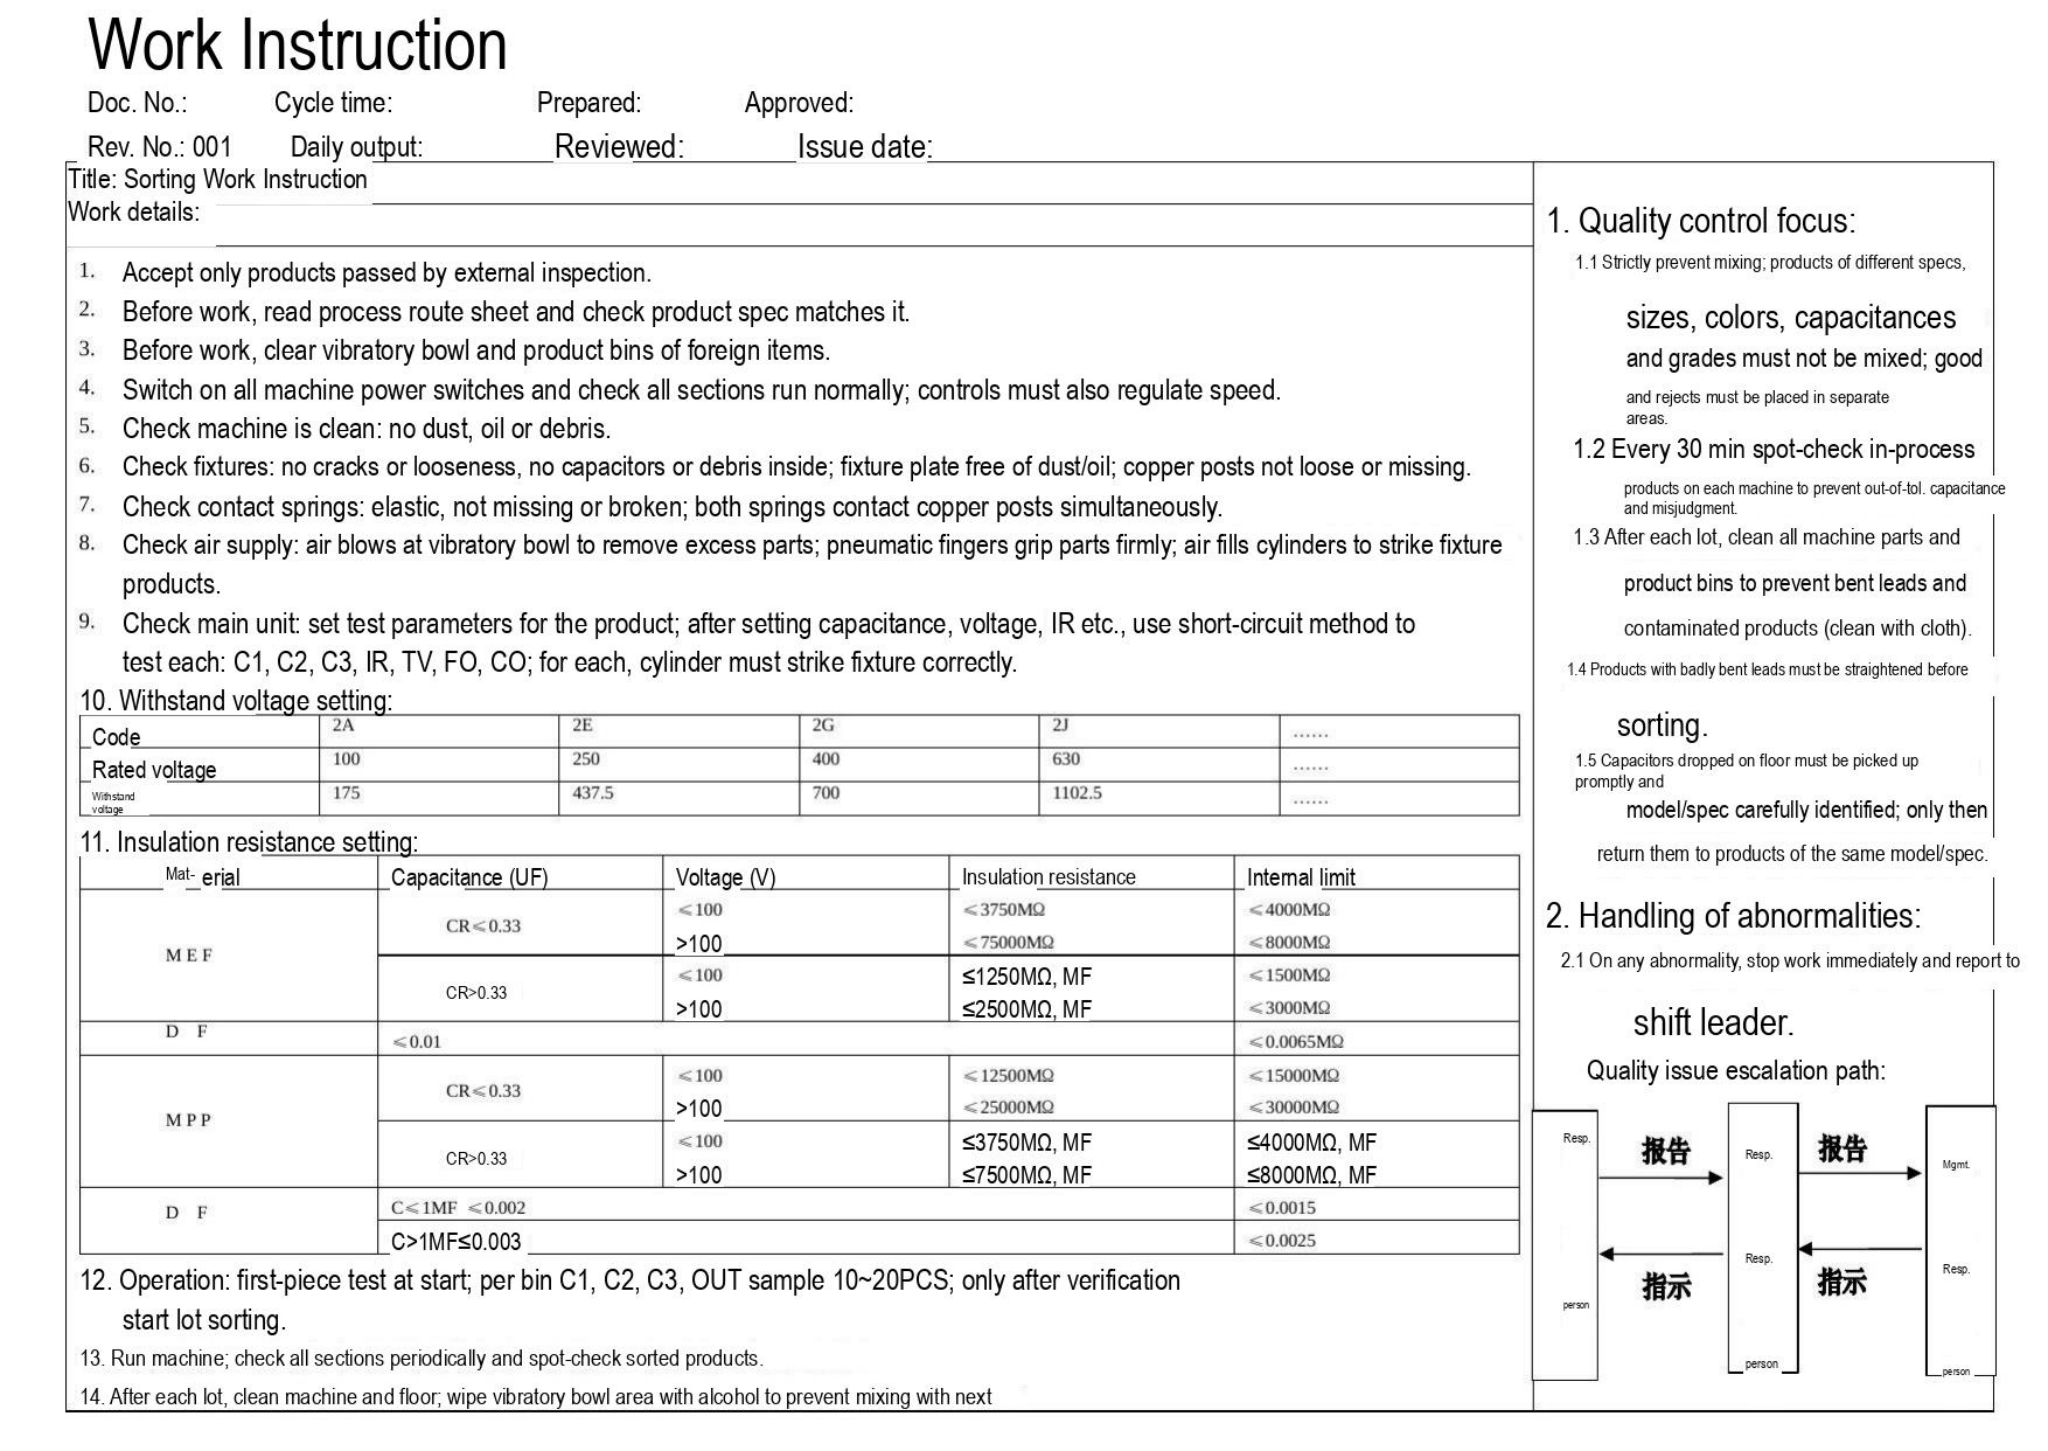Work Instruction

Doc. No.: Cycle time: Prepared: Approved:

Rev. No.: 001 Daily output: Reviewed: Issue date:

Title: Sorting Work Instruction

Work details:

1. Accept only products passed by external inspection.
2. Before work, read process route sheet and check product spec matches it.
3. Before work, clear vibratory bowl and product bins of foreign items.
4. Switch on all machine power switches and check all sections run normally; controls must also regulate speed.
5. Check machine is clean: no dust, oil or debris.
6. Check fixtures: no cracks or looseness, no capacitors or debris inside; fixture plate free of dust/oil; copper posts not loose or missing.
7. Check contact springs: elastic, not missing or broken; both springs contact copper posts simultaneously.
8. Check air supply: air blows at vibratory bowl to remove excess parts; pneumatic fingers grip parts firmly; air fills cylinders to strike fixture products.
9. Check main unit: set test parameters for the product; after setting capacitance, voltage, IR etc., use short-circuit method to test each: C1, C2, C3, IR, TV, FO, CO; for each, cylinder must strike fixture correctly.

10. Withstand voltage setting:

| Code | 2A | 2E | 2G | 2J | ...... |
|---|---|---|---|---|---|
| Rated voltage | 100 | 250 | 400 | 630 | ...... |
| Withstand voltage | 175 | 437.5 | 700 | 1102.5 | ...... |

11. Insulation resistance setting:

| Mat- erial | Capacitance (UF) | Voltage (V) | Insulation resistance | Internal limit |
|---|---|---|---|---|
| MEF | CR≤0.33 | ≤100 | ≤3750MΩ | ≤4000MΩ |
| | | >100 | ≤75000MΩ | ≤8000MΩ |
| | CR>0.33 | ≤100 | ≤1250MΩ, MF | ≤1500MΩ |
| | | >100 | ≤2500MΩ, MF | ≤3000MΩ |
| D F | ≤0.01 | | | ≤0.0065MΩ |
| MPP | CR≤0.33 | ≤100 | ≤12500MΩ | ≤15000MΩ |
| | | >100 | ≤25000MΩ | ≤30000MΩ |
| | CR>0.33 | ≤100 | ≤3750MΩ, MF | ≤4000MΩ, MF |
| | | >100 | ≤7500MΩ, MF | ≤8000MΩ, MF |
| D F | C≤1MF ≤0.002 | | | ≤0.0015 |
| | C>1MF≤0.003 | | | ≤0.0025 |

12. Operation: first-piece test at start; per bin C1, C2, C3, OUT sample 10~20PCS; only after verification start lot sorting.

13. Run machine; check all sections periodically and spot-check sorted products.

14. After each lot, clean machine and floor; wipe vibratory bowl area with alcohol to prevent mixing with next

1. Quality control focus:

1.1 Strictly prevent mixing; products of different specs, sizes, colors, capacitances and grades must not be mixed; good and rejects must be placed in separate areas.

1.2 Every 30 min spot-check in-process products on each machine to prevent out-of-tol. capacitance and misjudgment.

1.3 After each lot, clean all machine parts and product bins to prevent bent leads and contaminated products (clean with cloth).

1.4 Products with badly bent leads must be straightened before sorting.

1.5 Capacitors dropped on floor must be picked up promptly and model/spec carefully identified; only then return them to products of the same model/spec.

2. Handling of abnormalities:

2.1 On any abnormality, stop work immediately and report to shift leader.

Quality issue escalation path:

Resp. person

报告

指示

Resp. person

报告

指示

Mgmt. Resp. person
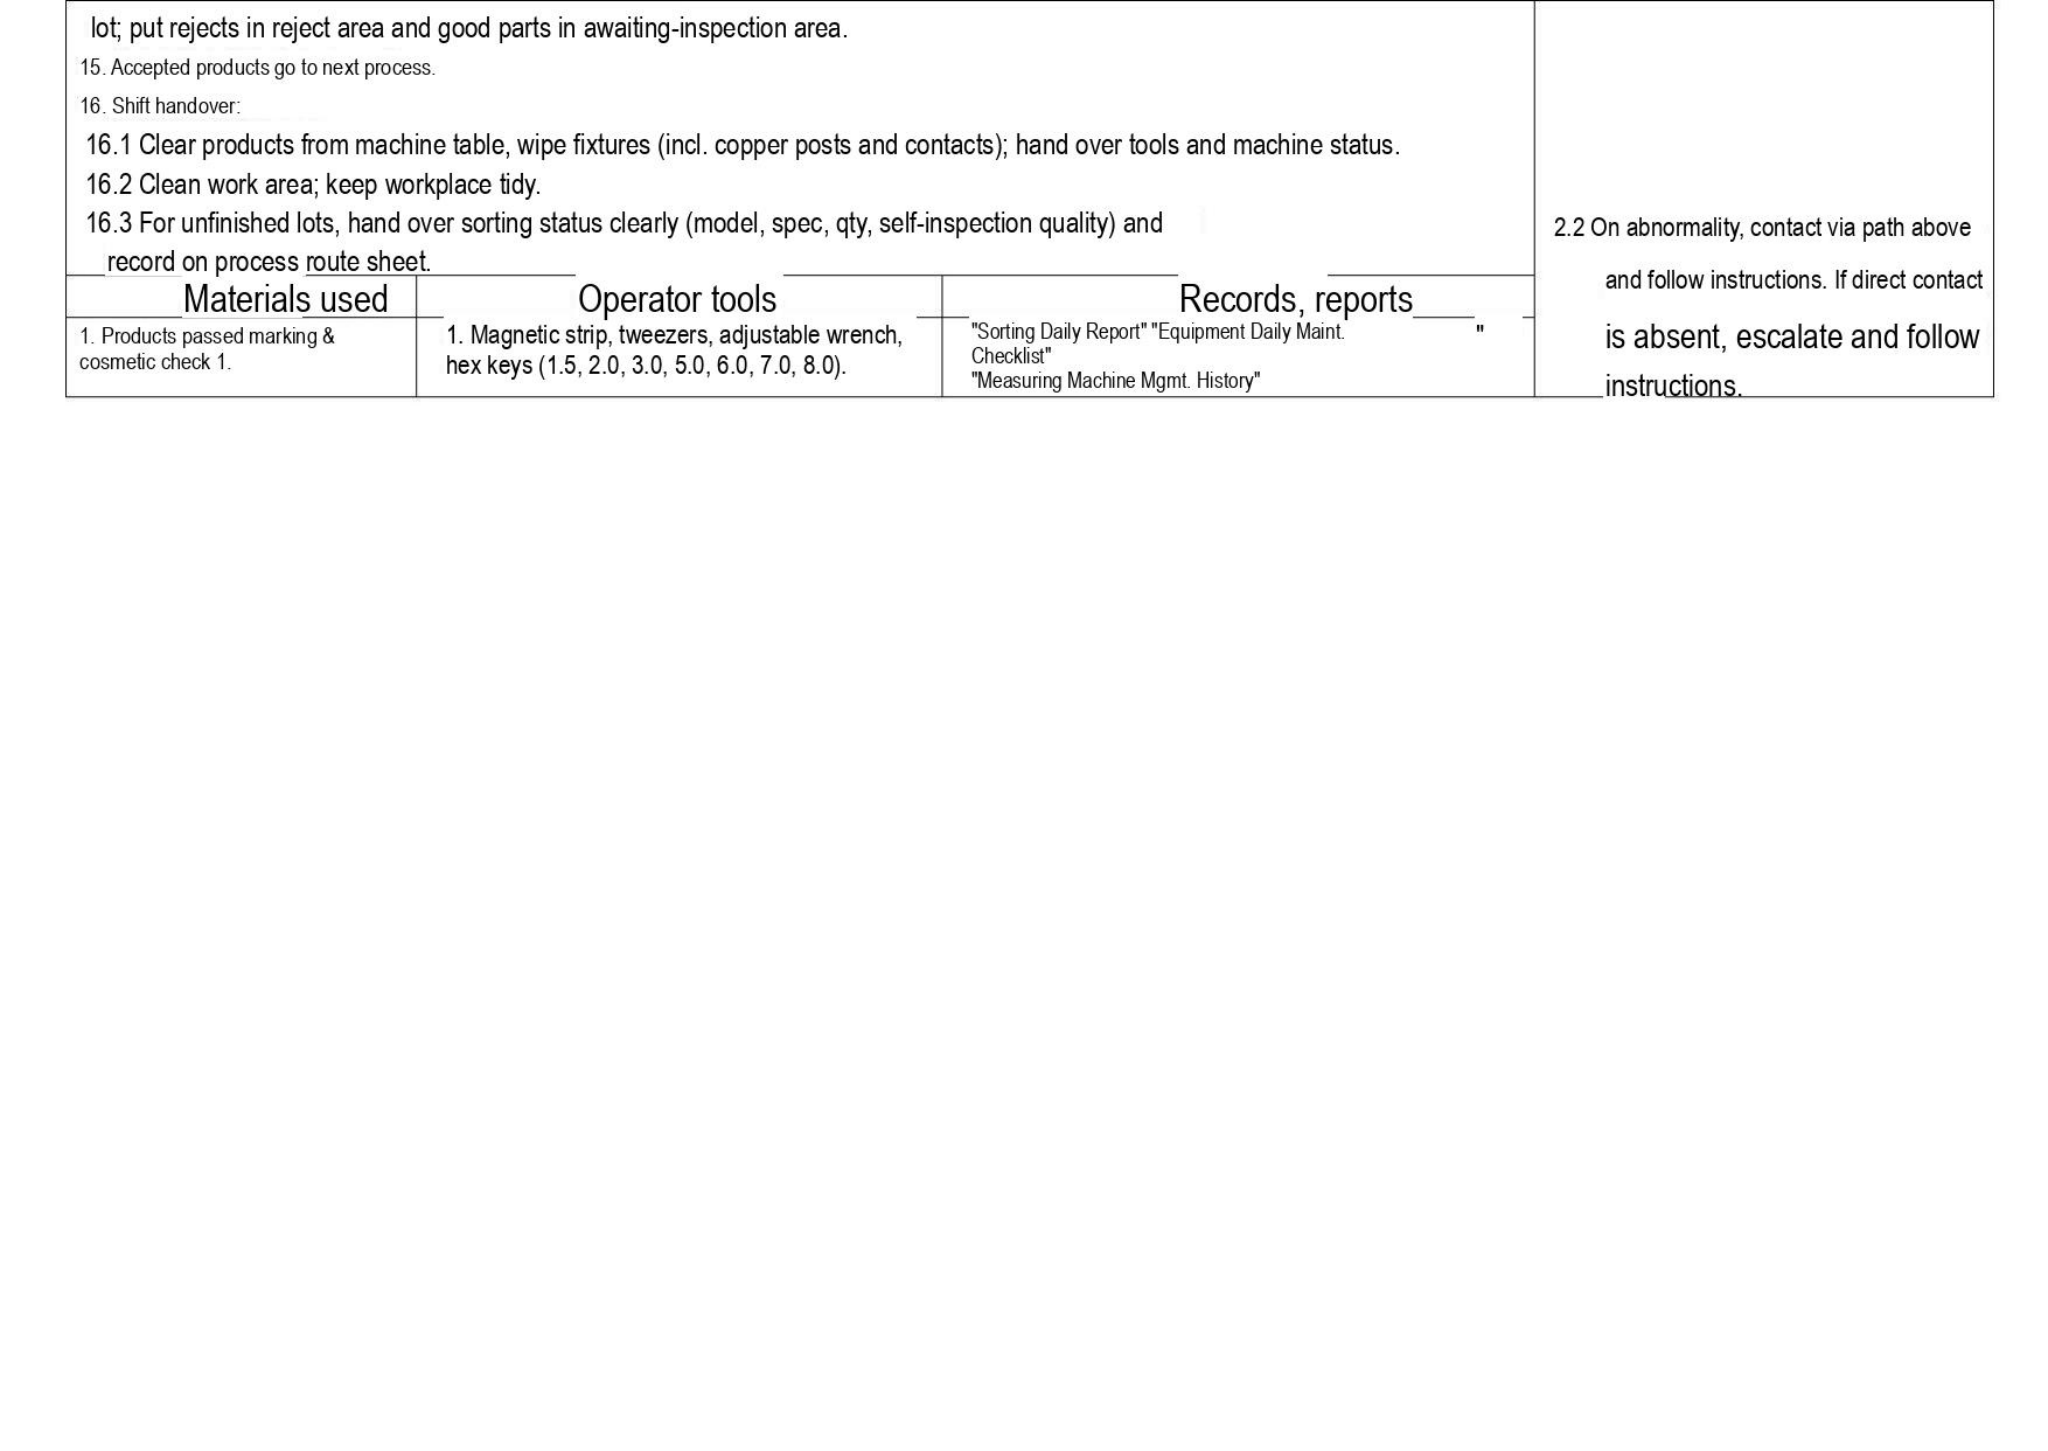lot; put rejects in reject area and good parts in awaiting-inspection area.
15. Accepted products go to next process.
16. Shift handover:
16.1 Clear products from machine table, wipe fixtures (incl. copper posts and contacts); hand over tools and machine status.
16.2 Clean work area; keep workplace tidy.
16.3 For unfinished lots, hand over sorting status clearly (model, spec, qty, self-inspection quality) and record on process route sheet.

| Materials used | Operator tools | Records, reports |
|---|---|---|
| 1. Products passed marking & cosmetic check 1. | 1. Magnetic strip, tweezers, adjustable wrench, hex keys (1.5, 2.0, 3.0, 5.0, 6.0, 7.0, 8.0). | "Sorting Daily Report" "Equipment Daily Maint. Checklist" "Measuring Machine Mgmt. History" |

2.2 On abnormality, contact via path above and follow instructions. If direct contact is absent, escalate and follow instructions.